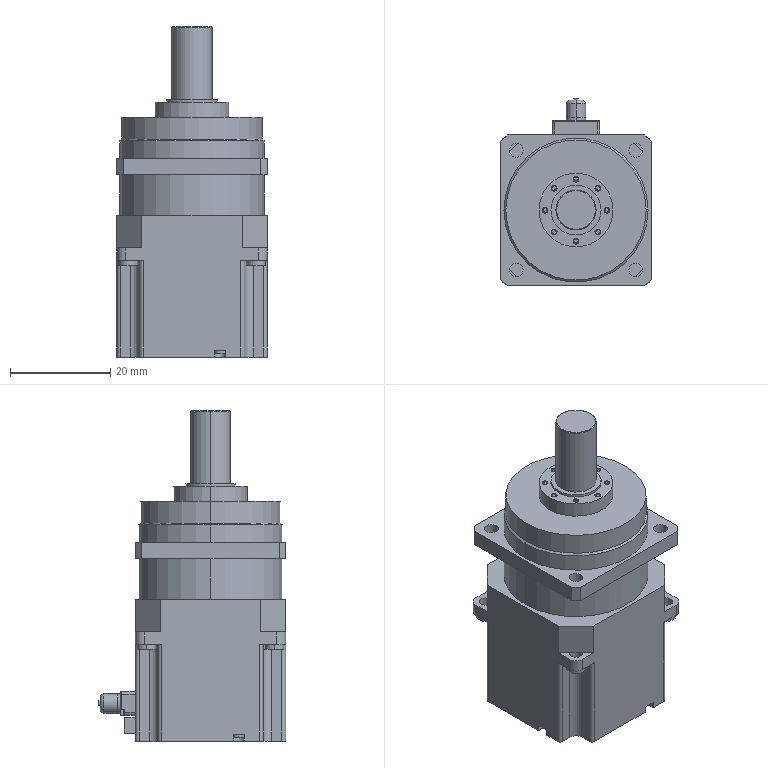Part | SolidWorks | features BaseBody 3, CombineBodies 1, Scale 1 | 1 solid | 426 faces | box 30 x 37.375 x 65.875 mm | volume 38357 mm3 | plane 291 | cylinder 123 | cone 4 | torus 4 | sphere 4 | commonest cylinder face diameters 1.012 x16 0.175 x8 1.187 x8 1.188 x8 1.5 x8 2.05 x8